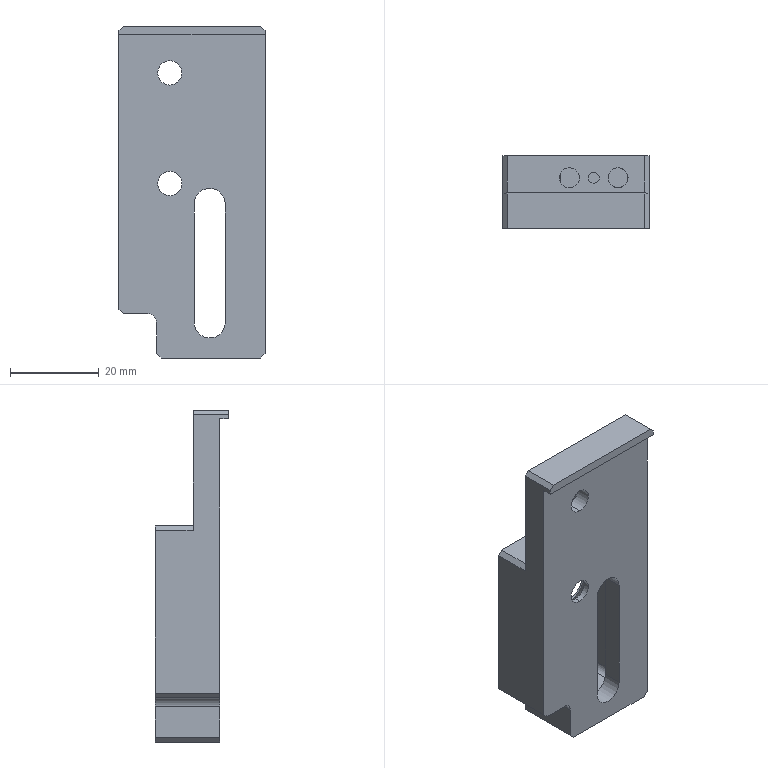Part | STEP file | 10000054304swp000-1 | 1 solid | 57 faces | box 33 x 16.5 x 75 mm | volume 16269 mm3 | plane 28 | cylinder 25 | cone 4 | commonest cylinder face diameters 2.5 x5 3 x4 4.5 x4 5.5 x4 4 x3 7 x3